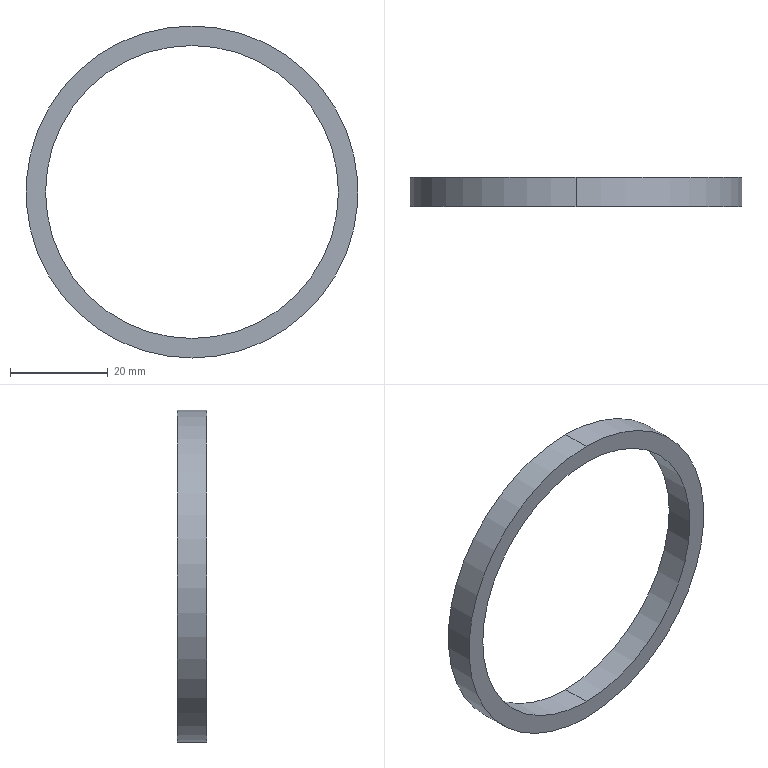Part | SolidWorks | features BaseBody 1 | 1 solid | 6 faces | box 68 x 6 x 68 mm | volume 4825 mm3 | cylinder 4 | plane 2 | commonest cylinder face diameters 60 x2 68 x2
STEP:
#1=CARTESIAN_POINT('',(0.,6.,30.));
#2=VERTEX_POINT('',#1);
#3=CARTESIAN_POINT('',(0.,6.,-30.));
#4=VERTEX_POINT('',#3);
#5=CARTESIAN_POINT('',(0.,6.,0.));
#6=DIRECTION('',(0.,-1.,0.));
#7=DIRECTION('',(0.,0.,-1.));
#8=AXIS2_PLACEMENT_3D('',#5,#6,#7);
#9=CIRCLE('',#8,30.);
#10=EDGE_CURVE('',#2,#4,#9,.T.);
#11=ORIENTED_EDGE('',*,*,#10,.F.);
#12=CARTESIAN_POINT('',(0.,0.,30.));
#13=VERTEX_POINT('',#12);
#14=CARTESIAN_POINT('',(0.,6.,30.));
#15=DIRECTION('',(0.,-1.,0.));
#16=VECTOR('',#15,1000.);
#17=LINE('',#14,#16);
#18=EDGE_CURVE('',#2,#13,#17,.T.);
#19=ORIENTED_EDGE('',*,*,#18,.T.);
#20=CARTESIAN_POINT('',(0.,0.,-30.));
#21=VERTEX_POINT('',#20);
#22=CARTESIAN_POINT('',(0.,0.,0.));
#23=DIRECTION('',(0.,1.,0.));
#24=DIRECTION('',(0.,0.,-1.));
#25=AXIS2_PLACEMENT_3D('',#22,#23,#24);
#26=CIRCLE('',#25,30.);
#27=EDGE_CURVE('',#21,#13,#26,.T.);
#28=ORIENTED_EDGE('',*,*,#27,.F.);
#29=CARTESIAN_POINT('',(0.,6.,-30.));
#30=DIRECTION('',(0.,-1.,0.));
#31=VECTOR('',#30,1000.);
#32=LINE('',#29,#31);
#33=EDGE_CURVE('',#4,#21,#32,.T.);
#34=ORIENTED_EDGE('',*,*,#33,.F.);
#35=EDGE_LOOP('',(#11,#19,#28,#34));
#36=FACE_OUTER_BOUND('',#35,.T.);
#37=CARTESIAN_POINT('',(0.,6.,0.));
#38=DIRECTION('',(0.,-1.,0.));
#39=DIRECTION('',(0.,0.,-1.));
#40=AXIS2_PLACEMENT_3D('',#37,#38,#39);
#41=CYLINDRICAL_SURFACE('',#40,30.);
#42=ADVANCED_FACE('',(#36),#41,.F.);
#43=CARTESIAN_POINT('',(0.,6.,34.));
#44=VERTEX_POINT('',#43);
#45=CARTESIAN_POINT('',(0.,6.,-34.));
#46=VERTEX_POINT('',#45);
#47=CARTESIAN_POINT('',(0.,6.,0.));
#48=DIRECTION('',(0.,1.,0.));
#49=DIRECTION('',(0.,0.,-1.));
#50=AXIS2_PLACEMENT_3D('',#47,#48,#49);
#51=CIRCLE('',#50,34.);
#52=EDGE_CURVE('',#44,#46,#51,.T.);
#53=ORIENTED_EDGE('',*,*,#52,.F.);
#54=CARTESIAN_POINT('',(0.,0.,34.));
#55=VERTEX_POINT('',#54);
#56=CARTESIAN_POINT('',(0.,6.,34.));
#57=DIRECTION('',(0.,-1.,0.));
#58=VECTOR('',#57,1000.);
#59=LINE('',#56,#58);
#60=EDGE_CURVE('',#44,#55,#59,.T.);
#61=ORIENTED_EDGE('',*,*,#60,.T.);
#62=CARTESIAN_POINT('',(0.,0.,-34.));
#63=VERTEX_POINT('',#62);
#64=CARTESIAN_POINT('',(0.,0.,0.));
#65=DIRECTION('',(0.,1.,0.));
#66=DIRECTION('',(0.,0.,-1.));
#67=AXIS2_PLACEMENT_3D('',#64,#65,#66);
#68=CIRCLE('',#67,34.);
#69=EDGE_CURVE('',#55,#63,#68,.T.);
#70=ORIENTED_EDGE('',*,*,#69,.T.);
#71=CARTESIAN_POINT('',(0.,6.,-34.));
#72=DIRECTION('',(0.,-1.,0.));
#73=VECTOR('',#72,1000.);
#74=LINE('',#71,#73);
#75=EDGE_CURVE('',#46,#63,#74,.T.);
#76=ORIENTED_EDGE('',*,*,#75,.F.);
#77=EDGE_LOOP('',(#53,#61,#70,#76));
#78=FACE_OUTER_BOUND('',#77,.T.);
#79=CARTESIAN_POINT('',(0.,6.,0.));
#80=DIRECTION('',(0.,-1.,0.));
#81=DIRECTION('',(0.,0.,-1.));
#82=AXIS2_PLACEMENT_3D('',#79,#80,#81);
#83=CYLINDRICAL_SURFACE('',#82,34.);
#84=ADVANCED_FACE('',(#78),#83,.T.);
#85=CARTESIAN_POINT('',(0.,6.,0.));
#86=DIRECTION('',(0.,-1.,0.));
#87=DIRECTION('',(0.,0.,-1.));
#88=AXIS2_PLACEMENT_3D('',#85,#86,#87);
#89=CIRCLE('',#88,30.);
#90=EDGE_CURVE('',#4,#2,#89,.T.);
#91=ORIENTED_EDGE('',*,*,#90,.T.);
#92=ORIENTED_EDGE('',*,*,#10,.T.);
#93=EDGE_LOOP('',(#91,#92));
#94=FACE_BOUND('',#93,.T.);
#95=CARTESIAN_POINT('',(0.,6.,0.));
#96=DIRECTION('',(0.,1.,0.));
#97=DIRECTION('',(0.,0.,-1.));
#98=AXIS2_PLACEMENT_3D('',#95,#96,#97);
#99=CIRCLE('',#98,34.);
#100=EDGE_CURVE('',#46,#44,#99,.T.);
#101=ORIENTED_EDGE('',*,*,#100,.T.);
#102=ORIENTED_EDGE('',*,*,#52,.T.);
#103=EDGE_LOOP('',(#101,#102));
#104=FACE_OUTER_BOUND('',#103,.T.);
#105=CARTESIAN_POINT('',(0.,6.,0.));
#106=DIRECTION('',(0.,1.,0.));
#107=DIRECTION('',(0.,0.,1.));
#108=AXIS2_PLACEMENT_3D('',#105,#106,#107);
#109=PLANE('',#108);
#110=ADVANCED_FACE('',(#94,#104),#109,.T.);
#111=ORIENTED_EDGE('',*,*,#18,.F.);
#112=ORIENTED_EDGE('',*,*,#90,.F.);
#113=ORIENTED_EDGE('',*,*,#33,.T.);
#114=CARTESIAN_POINT('',(0.,0.,0.));
#115=DIRECTION('',(0.,1.,0.));
#116=DIRECTION('',(0.,0.,-1.));
#117=AXIS2_PLACEMENT_3D('',#114,#115,#116);
#118=CIRCLE('',#117,30.);
#119=EDGE_CURVE('',#13,#21,#118,.T.);
#120=ORIENTED_EDGE('',*,*,#119,.F.);
#121=EDGE_LOOP('',(#111,#112,#113,#120));
#122=FACE_OUTER_BOUND('',#121,.T.);
#123=CARTESIAN_POINT('',(0.,6.,0.));
#124=DIRECTION('',(0.,-1.,0.));
#125=DIRECTION('',(0.,0.,-1.));
#126=AXIS2_PLACEMENT_3D('',#123,#124,#125);
#127=CYLINDRICAL_SURFACE('',#126,30.);
#128=ADVANCED_FACE('',(#122),#127,.F.);
#129=ORIENTED_EDGE('',*,*,#60,.F.);
#130=ORIENTED_EDGE('',*,*,#100,.F.);
#131=ORIENTED_EDGE('',*,*,#75,.T.);
#132=CARTESIAN_POINT('',(0.,0.,0.));
#133=DIRECTION('',(0.,1.,0.));
#134=DIRECTION('',(0.,0.,-1.));
#135=AXIS2_PLACEMENT_3D('',#132,#133,#134);
#136=CIRCLE('',#135,34.);
#137=EDGE_CURVE('',#63,#55,#136,.T.);
#138=ORIENTED_EDGE('',*,*,#137,.T.);
#139=EDGE_LOOP('',(#129,#130,#131,#138));
#140=FACE_OUTER_BOUND('',#139,.T.);
#141=CARTESIAN_POINT('',(0.,6.,0.));
#142=DIRECTION('',(0.,-1.,0.));
#143=DIRECTION('',(0.,0.,-1.));
#144=AXIS2_PLACEMENT_3D('',#141,#142,#143);
#145=CYLINDRICAL_SURFACE('',#144,34.);
#146=ADVANCED_FACE('',(#140),#145,.T.);
#147=ORIENTED_EDGE('',*,*,#27,.T.);
#148=ORIENTED_EDGE('',*,*,#119,.T.);
#149=EDGE_LOOP('',(#147,#148));
#150=FACE_BOUND('',#149,.T.);
#151=ORIENTED_EDGE('',*,*,#137,.F.);
#152=ORIENTED_EDGE('',*,*,#69,.F.);
#153=EDGE_LOOP('',(#151,#152));
#154=FACE_OUTER_BOUND('',#153,.T.);
#155=CARTESIAN_POINT('',(0.,0.,0.));
#156=DIRECTION('',(0.,1.,0.));
#157=DIRECTION('',(0.,0.,1.));
#158=AXIS2_PLACEMENT_3D('',#155,#156,#157);
#159=PLANE('',#158);
#160=ADVANCED_FACE('',(#150,#154),#159,.F.);
#161=CLOSED_SHELL('',(#42,#84,#110,#128,#146,#160));
#162=MANIFOLD_SOLID_BREP('',#161);
#163=CARTESIAN_POINT('',(0.,0.,0.));
#164=DIRECTION('',(0.,0.,1.));
#165=DIRECTION('',(1.,0.,0.));
#166=AXIS2_PLACEMENT_3D('',#163,#164,#165);
#167=(LENGTH_UNIT()NAMED_UNIT(*)SI_UNIT(.MILLI.,.METRE.));
#168=UNCERTAINTY_MEASURE_WITH_UNIT(LENGTH_MEASURE(0.00001),#167,'','');
#169=(NAMED_UNIT(*)PLANE_ANGLE_UNIT()SI_UNIT($,.RADIAN.));
#170=(NAMED_UNIT(*)SI_UNIT($,.STERADIAN.)SOLID_ANGLE_UNIT());
#171=(GEOMETRIC_REPRESENTATION_CONTEXT(3)GLOBAL_UNCERTAINTY_ASSIGNED_CONTEXT((#168))GLOBAL_UNIT_ASSIGNED_CONTEXT((#167,#169,#170))REPRESENTATION_CONTEXT('',''));
#172=ADVANCED_BREP_SHAPE_REPRESENTATION('',(#162,#166),#171);